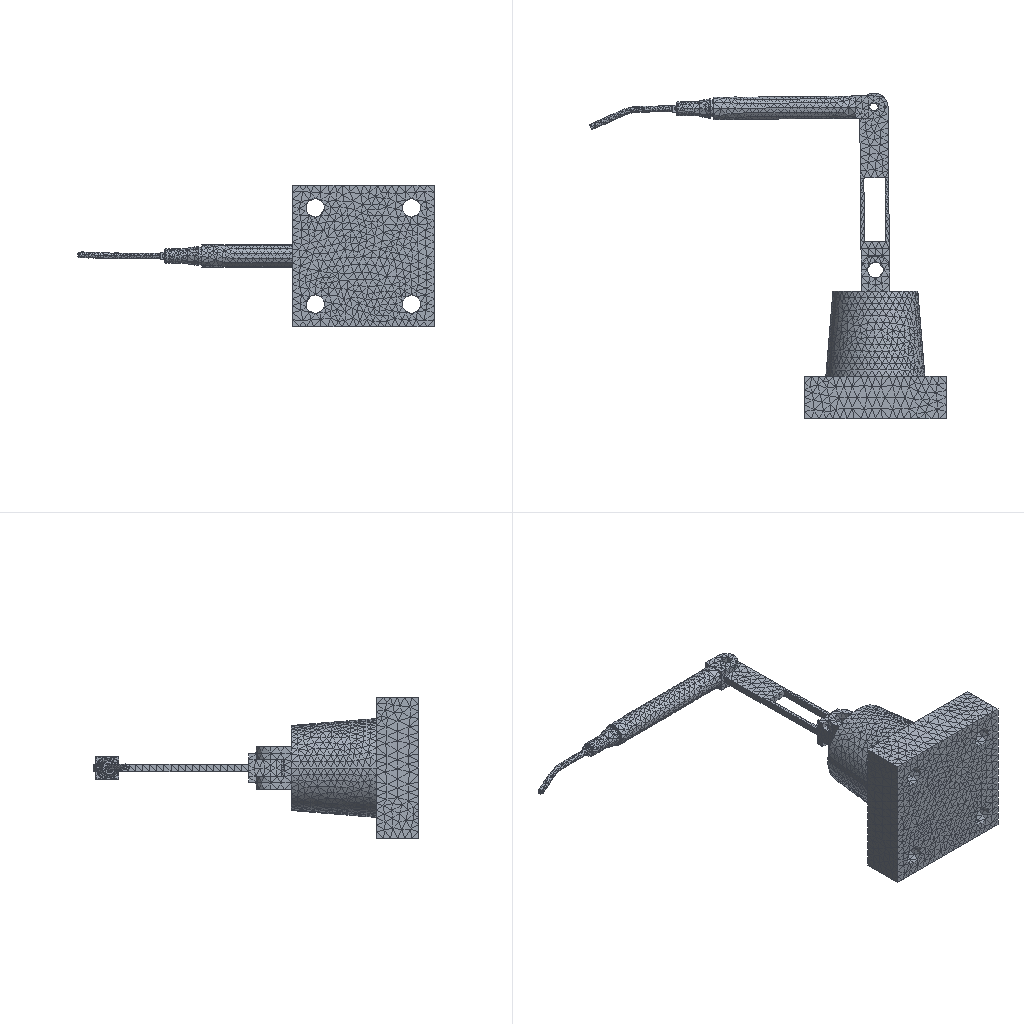Simulation study | ansys workbench
Set-up summary:
category,name,step,type,value,unit,region
solver,ansys_workbench
units,mm-N-s-tonne (MPa),,stated,"/units,MPA"
analysis,LS1,,static
load_step,LS1,LS1,static,nsubst=1; time=1
mesh,nodes,,,45184
mesh,elements,,,29144
element_type,SOLID187,,,28384
element_type,TARGE170,,,376
element_type,CONTA174,,,376
element_type,SURF154,,,8
material,Structural Steel,,E,200000,tonne s^-2 mm^-1
material,Structural Steel,,nu,0.3
material,Structural Steel,,density,7.85e-09,tonne mm^-3
material,Structural Steel,,conductivity,60.5,tonne mm s^-3 C^-1
material,Structural Steel,,specific_heat,4.34e+08,mm^2 s^-2 C^-1
material,Structural Steel,,cte,1.2e-05,C^-1
material,Structural Steel,,permeability,10000
material,Structural Steel,,resistivity,0.00017,ohm mm
material,"Aluminum Alloy , Wrought , 6061 , T6",,E,69040,tonne s^-2 mm^-1
material,"Aluminum Alloy , Wrought , 6061 , T6",,nu,0.33
material,"Aluminum Alloy , Wrought , 6061 , T6",,density,2.713e-09,tonne mm^-3
material,"Aluminum Alloy , Wrought , 6061 , T6",,conductivity,155.3,tonne mm s^-3 C^-1
material,"Aluminum Alloy , Wrought , 6061 , T6",,specific_heat,9.157e+08,mm^2 s^-2 C^-1
material,"Aluminum Alloy , Wrought , 6061 , T6",,cte,2.278e-05,C^-1
load,Define Force Using Surface Effect Elements,LS1,surface-effect pres face 2,-1.02,,SURF154 #11
bc,Fixed Supports,model,fixed,[dofs=ALL],,_FIXEDSU
bc,Frictionless Supports Y,model,fixed,[dofs=UY],,_FRICSUY
contact,Contact Region,,bonded (always),element=CONTA174
contact,Contact Region 2,,bonded (always),element=CONTA174
contact,Contact Region 3,,bonded (always),element=CONTA174
named_set,_FIXEDSU,,node,312
named_set,_FRICSUY,,node,1585
Ansys APDL input file, long lists of numbers shortened:
/batch
/config,noeldb,1     ! force off writing results to database
*get,_wallstrt,active,,time,wall
! ANSYS input file written by Workbench version 2021 R1
! File used for geometry attach:
/title,wbnew--____ (B5)
! ****** Begin Custom Load Command Snippet ******
/COM, ACT Extensions:
/COM,     LSDYNA, 2021.1
/COM,
! ****** End   Custom Load Command Snippet ******
*DIM,_wb_ProjectScratch_dir,string,248
_wb_ProjectScratch_dir(1) = ''
*DIM,_wb_SolverFiles_dir,string,248
_wb_SolverFiles_dir(1) = ''
*DIM,_wb_userfiles_dir,string,248
_wb_userfiles_dir(1) = ''
/com,--- Data in consistent NMM units. See Solving Units in the help system for more information.
/units,MPA
/nopr
/wb,file,start              !  signify a WB generated input file
/prep7
! Turn off shape checking because checks already performed inside WB mesher.
! See help system for more information.
SHPP,OFF,,NOWARN
/nolist
etcon,set             ! allow ANSYS to choose best KEYOP's for 180x elements, resets any applicable keyopt to MAPDL defaults
/com,*********** Nodes for the whole assembly ***********
nblock,3,,49702
(1i9,3e20.9e3)
        1    -5.999740841E+00     1.049442340E+02     6.000000000E+00
! (45183 more lines like these left out)
-1
/wb,elem,start            !  set before creation of elements
/com,*********** Elements for Body 1 "__|____1" ***********
et,1,187
eblock,19,solid,,19124
(19i9)
        1        1        1        1        0        0        0        0       10        0     9261    17255    17810    19772    18810    31043    34585    31047    31045
! (38247 more lines like these left out)
-1
/com,*********** Elements for Body 2 "__|____-____3" ***********
et,2,187
eblock,19,solid,,917
(19i9)
        2        2        2        2        0        0        0        0       10        0        1      252      372      267      265     1653     1696     1652     1651
! (1833 more lines like these left out)
-1
/com,*********** Elements for Body 3 "____|____10" ***********
et,3,187
eblock,19,solid,,5842
(19i9)
        3        3        3        3        0        0        0        0       10        0     3419     6840     7705     6857     7188    11511    11618    11504    11510
! (11683 more lines like these left out)
-1
/com,*********** Elements for Body 4 "__1|____1" ***********
et,4,187
eblock,19,solid,,2501
(19i9)
        4        4        4        4        0        0        0        0       10        0      918     2645     2662     2706     2705     6261     6328     6267     6266
! (5001 more lines like these left out)
-1
/wb,elem,end               !  done creating elements
/com,*********** Send User Defined Coordinate System(s) ***********
csys,0
toffst,273.15,  ! Temperature offset from absolute zero
/com,*********** Set Reference Temperature ***********
tref,22.
/wb,mat,start              !  starting to send materials
/com,*********** Send Materials ***********
Temperature = 'TEMP' ! Temperature
MP,DENS,1,7.85e-09,	! tonne mm^-3
MP,ALPX,1,1.2e-05,	! C^-1
MP,C,1,434000000,	! mm^2 s^-2 C^-1
MP,KXX,1,60.5,	! tonne mm s^-3 C^-1
MP,RSVX,1,0.00017,	! ohm mm
MP,EX,1,200000,	! tonne s^-2 mm^-1
MP,NUXY,1,0.3,
MP,MURX,1,10000,
Temperature = 'TEMP' ! Temperature
MP,DENS,2,2.713e-09,	! tonne mm^-3
MP,EX,2,69040,	! tonne s^-2 mm^-1
MP,NUXY,2,0.33,
MP,ALPX,2,2.278e-05,	! C^-1
MP,KXX,2,155.3,	! tonne mm s^-3 C^-1
MP,C,2,915700000,	! mm^2 s^-2 C^-1
Temperature = 'TEMP' ! Temperature
MP,DENS,3,2.713e-09,	! tonne mm^-3
MP,EX,3,69040,	! tonne s^-2 mm^-1
MP,NUXY,3,0.33,
MP,ALPX,3,2.278e-05,	! C^-1
MP,KXX,3,155.3,	! tonne mm s^-3 C^-1
MP,C,3,915700000,	! mm^2 s^-2 C^-1
Temperature = 'TEMP' ! Temperature
MP,DENS,4,2.713e-09,	! tonne mm^-3
MP,EX,4,69040,	! tonne s^-2 mm^-1
MP,NUXY,4,0.33,
MP,ALPX,4,2.278e-05,	! C^-1
MP,KXX,4,155.3,	! tonne mm s^-3 C^-1
MP,C,4,915700000,	! mm^2 s^-2 C^-1
/wb,mat,end                !  done sending materials
!************************* Model Summary ********************
!__|____1,	结构钢,	matid,	1
!__|____-____3,	铝合金，锻造，6061，T6,	matid,	2
!____|____10,	铝合金，锻造，6061，T6,	matid,	3
!__1|____1,	铝合金，锻造，6061，T6,	matid,	4
!************************* End Model Summary ********************
! get the diagonal of the bounding box. Needed later for other things
*get,_xmin,node,,mnloc,x
*get,_ymin,node,,mnloc,y
*get,_zmin,node,,mnloc,z
*get,_xmax,node,,mxloc,x
*get,_ymax,node,,mxloc,y
*get,_zmax,node,,mxloc,z
_ASMDIAG=(_xmax-_xmin)*(_xmax-_xmin)+(_ymax-_ymin)*(_ymax-_ymin)+(_zmax-_zmin)*(_zmax-_zmin)
_ASMDIAG=SQRT(_ASMDIAG)
/wb,contact,start          !  starting to send contact
/com,*********** Create Contact "接触区域" ***********
/com,            Real Constant Set For Above Contact Is 6 & 5
*set,tid,6
*set,cid,5
r,tid
r,cid
et,tid,170
et,cid,174
eblock,10,,,104
(15i9)
    35303        6        6        6        0    15763    15761    15770    15770    21813    21814    15770    21820
! (103 more lines like these left out)
-1
eblock,10,,,104
(15i9)
    35407        5        5        5        0    15763    15761    15770    15770    21813    21814    15770    21820
! (103 more lines like these left out)
-1
eblock,10,,,98
(15i9)
    35511        5        6        5        0      107      158      150      150     1037     1255      150     1036
! (97 more lines like these left out)
-1
eblock,10,,,98
(15i9)
    35609        6        5        6        0      107      158      150      150     1037     1255      150     1036
! (97 more lines like these left out)
-1
keyo,cid,8,2               ! auto create asymmetric contact (from Program Controlled setting)
keyo,cid,10,0              ! adjust contact stiffness each NR iteration (from Program Controlled setting)
keyo,cid,12,5              ! bonded always
keyo,cid,18,1              ! small sliding turned on by application
keyo,cid,2,0               ! augmented Lagrange (from Program Controlled setting)
keyo,cid,4,0               ! on Gauss point (from Program Controlled setting)
keyo,cid,9,1               ! ignore initial gaps/penetration
keyo,cid,7,0               ! No Prediction
rmod,tid,3,10.      ! FKN
rmod,tid,5,0.       ! ICONT
rmod,tid,6,0.       ! PINB
rmod,tid,10,0.      ! CNOF
rmod,tid,12,0.      ! FKT
rmod,tid,36,34      ! WB DSID
rmod,cid,3,10.      ! FKN
rmod,cid,5,0.       ! ICONT
rmod,cid,6,0.       ! PINB
rmod,cid,10,0.      ! CNOF
rmod,cid,12,0.      ! FKT
rmod,cid,36,34      ! WB DSID
/com,*********** Create Contact "接触区域 2" ***********
/com,            Real Constant Set For Above Contact Is 8 & 7
*set,tid,8
*set,cid,7
r,tid
r,cid
et,tid,170
et,cid,174
eblock,10,,,102
(15i9)
    35707        8        8        8        0      109      108      130      130     1039     1041      130     1047
! (101 more lines like these left out)
-1
eblock,10,,,102
(15i9)
    35809        7        7        7        0      109      108      130      130     1039     1041      130     1047
! (101 more lines like these left out)
-1
eblock,10,,,56
(15i9)
    35911        7        8        7        0     2186     2183     2165     2165     3825     3753     2165     3754
! (55 more lines like these left out)
-1
eblock,10,,,56
(15i9)
    35967        8        7        8        0     2186     2183     2165     2165     3825     3753     2165     3754
! (55 more lines like these left out)
-1
keyo,cid,8,2               ! auto create asymmetric contact (from Program Controlled setting)
keyo,cid,10,0              ! adjust contact stiffness each NR iteration (from Program Controlled setting)
keyo,cid,12,5              ! bonded always
keyo,cid,18,1              ! small sliding turned on by application
keyo,cid,2,0               ! augmented Lagrange (from Program Controlled setting)
keyo,cid,4,0               ! on Gauss point (from Program Controlled setting)
keyo,cid,9,1               ! ignore initial gaps/penetration
keyo,cid,7,0               ! No Prediction
rmod,tid,3,10.      ! FKN
rmod,tid,5,0.       ! ICONT
rmod,tid,6,0.       ! PINB
rmod,tid,10,0.      ! CNOF
rmod,tid,12,0.      ! FKT
rmod,tid,36,37      ! WB DSID
rmod,cid,3,10.      ! FKN
rmod,cid,5,0.       ! ICONT
rmod,cid,6,0.       ! PINB
rmod,cid,10,0.      ! CNOF
rmod,cid,12,0.      ! FKT
rmod,cid,36,37      ! WB DSID
/com,*********** Create Contact "接触区域 3" ***********
/com,            Real Constant Set For Above Contact Is 10 & 9
*set,tid,10
*set,cid,9
r,tid
r,cid
et,tid,170
et,cid,174
eblock,10,,,8
(15i9)
    36023       10       10       10        0     6496     6998     6497     6497     8971     8977     6497     8968
! (7 more lines like these left out)
-1
eblock,10,,,8
(15i9)
    36031        9        9        9        0     6496     6998     6497     6497     8971     8977     6497     8968
! (7 more lines like these left out)
-1
eblock,10,,,8
(15i9)
    36039        9       10        9        0     2197     2198     2483     2483     3929     3938     2483     3933
! (7 more lines like these left out)
-1
eblock,10,,,8
(15i9)
    36047       10        9       10        0     2197     2198     2483     2483     3929     3938     2483     3933
! (7 more lines like these left out)
-1
keyo,cid,8,2               ! auto create asymmetric contact (from Program Controlled setting)
keyo,cid,10,0              ! adjust contact stiffness each NR iteration (from Program Controlled setting)
keyo,cid,12,5              ! bonded always
keyo,cid,18,1              ! small sliding turned on by application
keyo,cid,2,0               ! augmented Lagrange (from Program Controlled setting)
keyo,cid,4,0               ! on Gauss point (from Program Controlled setting)
keyo,cid,9,1               ! ignore initial gaps/penetration
keyo,cid,7,0               ! No Prediction
rmod,tid,3,10.      ! FKN
rmod,tid,5,0.       ! ICONT
rmod,tid,6,0.       ! PINB
rmod,tid,10,0.      ! CNOF
rmod,tid,12,0.      ! FKT
rmod,tid,36,40      ! WB DSID
rmod,cid,3,10.      ! FKN
rmod,cid,5,0.       ! ICONT
rmod,cid,6,0.       ! PINB
rmod,cid,10,0.      ! CNOF
rmod,cid,12,0.      ! FKT
rmod,cid,36,40      ! WB DSID
nsel,all
esel,all
/wb,contact,end            !  done creating contacts
/golist
/wb,load,start             !  starting to send loads
/com,*********** Fixed Supports ***********
CMBLOCK,_FIXEDSU,NODE,      312
(8i10)
     15519     15520     15521     15522     15523     15524     15525     15526
! (38 more lines like these left out)
cmsel,s,_FIXEDSU
d,all,all
nsel,all
/com,********* Frictionless Supports Y *********
CMBLOCK,_FRICSUY,NODE,     1585
(8i10)
     15530     15531     15532     15533     15534     15535     15570     15571
! (198 more lines like these left out)
cmsel,s,_FRICSUY
d,all,uy,0
nsel,all
/com,*********** Define Force Using Surface Effect Elements ***********
local,12,0,0.,0.,0.,0.,0.,0.
csys,0
et,11,154
eblock,10,,,8
(15i9)
    36055       11       11       11       12     2197     2198     2483     2483     3929     3938     2483     3933
! (7 more lines like these left out)
-1
esel,s,type,,11
keyop,11,2,1                ! Apply load in local coordinate system
keyop,11,7,1                ! Use original area so load is constant in large deformation
esel,all
/gst,on,on
fini
*get,_numnode,node,0,count
*get,_numelem,elem,0,count
*get, _MAXELEMNUM, elem, 0, NUM, MAX
*get, _MAXNODENUM, node, 0, NUM, MAX
*get, _MAXELEMTYPE, etyp, 0, NUM, MAX
*get, _MAXREALCONST, real, 0, NUM, MAX
/go
/wb,load,end               !  done creating loads
/com,--- Number of total nodes = %_numnode%
/com,--- Number of contact elements = 760
/com,--- Number of spring elements = 0
/com,--- Number of bearing elements = 0
/com,--- Number of solid elements = 28384
/com,--- Number of condensed parts = 0
/com,--- Number of total elements = %_numelem%
*get,_wallbsol,active,,time,wall
/com,****************************************************************************
/com,*************************    SOLUTION       ********************************
/com,****************************************************************************
/solu
antype,0                   ! static analysis
_thickRatio=0.75    ! Ratio of thick parts in the model
eqsl,pcg,1e-8,,,,,,1
cntr,print,1               ! print out contact info and also make no initial contact an error
dmpoption,emat,no             ! Don't combine emat file for DANSYS
dmpoption,esav,no             ! Don't combine esav file for DANSYS
nldiag,cont,iter           ! print out contact info each equilibrium iteration
rescontrol,,none                 ! Do not keep any restart files
/com,****************************************************
/com,******************* SOLVE FOR LS 1 OF 1 ****************
esel,s,type,,11
nsle
sfe,all,1,pres,1,0.
sfe,all,2,pres,1,-1.02
sfe,all,3,pres,1,0.
nsel,all
esel,all
/nopr
/gopr
/nolist
nsub,1,1,1
time,1.
outres,erase
outres,all,none
outres,nsol,all,
outres,rsol,all
outres,eangl,all
outres,etmp,all
outres,veng,all
outres,strs,all,
outres,epel,all,
outres,eppl,all,
outres,cont,all,
! *********** WB SOLVE COMMAND ***********
! check interactive state
*get,ANSINTER_,active,,int
*if,ANSINTER_,ne,0,then
/eof
*endif
solve
/com *************** Write FE CONNECTORS *********
CEWRITE,file,ce,,INTE
/com,****************************************************
/com,*************** FINISHED SOLVE FOR LS 1 *************
*get,_wallasol,active,,time,wall
/nopr
*get,_numnode,node,0,count
*get,_numelem,elem,0,count
*get, _MAXELEMNUM, elem, 0, NUM, MAX
*get, _MAXNODENUM, node, 0, NUM, MAX,,,INTERNAL
*get, _MAXELEMTYPE, etyp, 0, NUM, MAX
*get, _MAXREALCONST, real, 0, NUM, MAX
/gopr
*get,_PCGITER,active,,solu,cgiter
/post1
xmlo,ENCODING,ISO-8859-1
xmlo,parm
/xml,parm,xml
fini
/gopr
*get,_walldone,active,,time,wall
_preptime=(_wallbsol-_wallstrt)*3600
_solvtime=(_wallasol-_wallbsol)*3600
_posttime=(_walldone-_wallasol)*3600
_totaltim=(_walldone-_wallstrt)*3600
*get,_dlbratio,active,0,solu,dlbr
*get,_combtime,active,0,solu,comb
/com,--- Total number of nodes = %_numnode%
/com,--- Total number of elements = %_numelem%
/com,--- Element load balance ratio = %_dlbratio%
/com,--- Time to combine distributed files = %_combtime%
/wb,file,end               ! done with WB generated input
Results summary:
result,analyses[0].index,,,1
result,analyses[0].system,,,SYS-1
result,analyses[0].deck,,,deck.dat
result,analyses[0].solve_status,,,completed
result,analyses[0].analysis_type,,,static
result,analyses[0].physics,,,mechanical
result,analyses[0].unit_system,,,"NMM: mm, ton, N, s, mV, mA, degC"
result,analyses[0].n_sets,,,1
result,analyses[0].load_steps[0].set,set=1,,1
result,analyses[0].load_steps[0].time_or_freq,set=1,,1
result,analyses[0].load_steps[0].max_displacement_magnitude,set=1,,1.866
result,analyses[0].load_steps[0].max_von_mises_nodal,set=1,,157.076
result,analyses[0].load_steps[0].reaction_force_sum_xyz[1],set=1,,-1.12386e-08
result,analyses[0].load_steps[0].reaction_force_sum_xyz[2],set=1,,100
result,analyses[0].load_steps[0].reaction_force_sum_xyz[3],set=1,,5.97281e-08
result,geometry_export[0][0],,,.step
result,geometry_export[0][1],,,ok
result,geometry_export[0][2],,,4